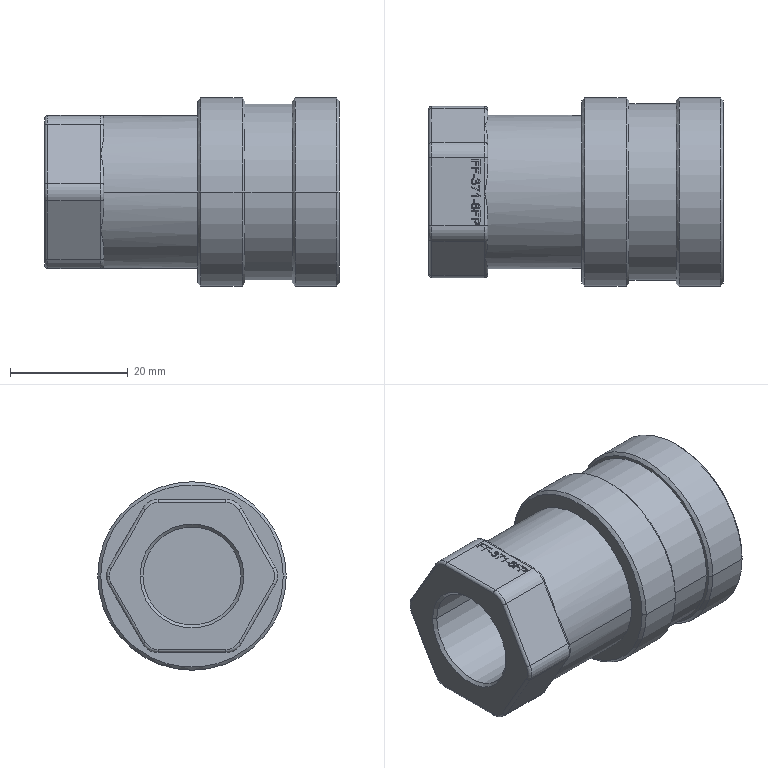Part | STEP file | 4-20.sldasm-Part-139 | 1 solid | 216 faces | box 50 x 32 x 32 mm | volume 24309 mm3 | plane 93 | spline 48 | cylinder 43 | cone 18 | torus 14 | commonest cylinder face diameters 1 x18 6 x7 32 x4 13 x2 14 x2 16.66 x2